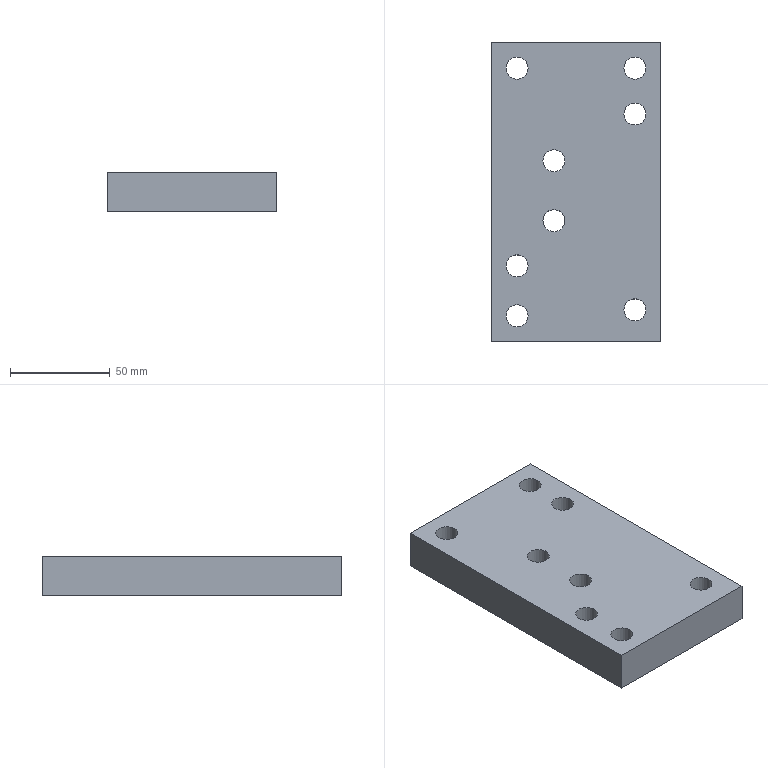Part | STEP file | 106_id3178_x_t | 1 solid | 14 faces | box 85 x 150 x 20 mm | volume 239795 mm3 | cylinder 8 | plane 6 | commonest cylinder face diameters 11 x8
STEP:
#1=CARTESIAN_POINT('',(0.,0.,0.));
#2=DIRECTION('',(0.,0.,1.));
#3=DIRECTION('',(1.,0.,0.));
#4=AXIS2_PLACEMENT_3D('',#1,#2,#3);
#5=CARTESIAN_POINT('',(-565.5,-67.,105.));
#6=VERTEX_POINT('',#5);
#7=CARTESIAN_POINT('',(-571.,-67.,105.));
#8=DIRECTION('',(0.,0.,-1.));
#9=DIRECTION('',(1.,0.,0.));
#10=AXIS2_PLACEMENT_3D('',#7,#8,#9);
#11=CIRCLE('',#10,5.5);
#12=CARTESIAN_POINT('',(-571.,-67.,90.));
#13=DIRECTION('',(0.,0.,1.));
#14=DIRECTION('',(-1.,0.,0.));
#15=AXIS2_PLACEMENT_3D('',#12,#13,#14);
#16=CYLINDRICAL_SURFACE('',#15,5.5);
#17=CARTESIAN_POINT('',(9.425,15.));
#18=DIRECTION('',(-1.,0.));
#19=VECTOR('',#18,1.);
#20=LINE('',#17,#19);
#21=(GEOMETRIC_REPRESENTATION_CONTEXT(2)PARAMETRIC_REPRESENTATION_CONTEXT()REPRESENTATION_CONTEXT('',''));
#22=DEFINITIONAL_REPRESENTATION('',(#20),#21);
#23=PCURVE('',#16,#22);
#24=CARTESIAN_POINT('',(-532.5,-4.,105.));
#25=DIRECTION('',(0.,0.,1.));
#26=DIRECTION('',(0.,-1.,0.));
#27=AXIS2_PLACEMENT_3D('',#24,#25,#26);
#28=PLANE('',#27);
#29=CARTESIAN_POINT('',(63.,-33.));
#30=CARTESIAN_POINT('',(72.526,-33.));
#31=CARTESIAN_POINT('',(67.763,-41.25));
#32=CARTESIAN_POINT('',(63.,-49.5));
#33=CARTESIAN_POINT('',(58.237,-41.25));
#34=CARTESIAN_POINT('',(53.474,-33.));
#35=CARTESIAN_POINT('',(63.,-33.));
#36=(BOUNDED_CURVE()B_SPLINE_CURVE(2,(#29,#30,#31,#32,#33,#34,#35),.UNSPECIFIED.,.T.,.F.)B_SPLINE_CURVE_WITH_KNOTS((1,2,2,2,2,1),(-2.094,0.,2.094,4.189,6.283,8.378),.UNSPECIFIED.)CURVE()GEOMETRIC_REPRESENTATION_ITEM()RATIONAL_B_SPLINE_CURVE((1.,0.5,1.,0.5,1.,0.5,1.))REPRESENTATION_ITEM(''));
#37=(GEOMETRIC_REPRESENTATION_CONTEXT(2)PARAMETRIC_REPRESENTATION_CONTEXT()REPRESENTATION_CONTEXT('',''));
#38=DEFINITIONAL_REPRESENTATION('',(#36),#37);
#39=PCURVE('',#28,#38);
#40=SURFACE_CURVE('',#11,(#23,#39),.PCURVE_S1.);
#41=EDGE_CURVE('',#6,#6,#40,.T.);
#42=ORIENTED_EDGE('',*,*,#41,.T.);
#43=CARTESIAN_POINT('',(-565.5,-67.,85.));
#44=VERTEX_POINT('',#43);
#45=CARTESIAN_POINT('',(-565.5,-67.,85.));
#46=CARTESIAN_POINT('',(-565.5,-67.,105.));
#47=B_SPLINE_CURVE_WITH_KNOTS('',1,(#45,#46),.UNSPECIFIED.,.F.,.F.,(2,2),(-5.,15.),.PIECEWISE_BEZIER_KNOTS.);
#48=CARTESIAN_POINT('',(3.142,0.));
#49=DIRECTION('',(0.,1.));
#50=VECTOR('',#49,1.);
#51=LINE('',#48,#50);
#52=(GEOMETRIC_REPRESENTATION_CONTEXT(2)PARAMETRIC_REPRESENTATION_CONTEXT()REPRESENTATION_CONTEXT('',''));
#53=DEFINITIONAL_REPRESENTATION('',(#51),#52);
#54=PCURVE('',#16,#53);
#55=CARTESIAN_POINT('',(9.425,0.));
#56=DIRECTION('',(0.,1.));
#57=VECTOR('',#56,1.);
#58=LINE('',#55,#57);
#59=(GEOMETRIC_REPRESENTATION_CONTEXT(2)PARAMETRIC_REPRESENTATION_CONTEXT()REPRESENTATION_CONTEXT('',''));
#60=DEFINITIONAL_REPRESENTATION('',(#58),#59);
#61=PCURVE('',#16,#60);
#62=SEAM_CURVE('',#47,(#54,#61),.PCURVE_S1.);
#63=EDGE_CURVE('',#44,#6,#62,.T.);
#64=ORIENTED_EDGE('',*,*,#63,.F.);
#65=CARTESIAN_POINT('',(-571.,-67.,85.));
#66=DIRECTION('',(0.,0.,1.));
#67=DIRECTION('',(-1.,0.,0.));
#68=AXIS2_PLACEMENT_3D('',#65,#66,#67);
#69=CIRCLE('',#68,5.5);
#70=CARTESIAN_POINT('',(0.,-5.));
#71=DIRECTION('',(1.,0.));
#72=VECTOR('',#71,1.);
#73=LINE('',#70,#72);
#74=(GEOMETRIC_REPRESENTATION_CONTEXT(2)PARAMETRIC_REPRESENTATION_CONTEXT()REPRESENTATION_CONTEXT('',''));
#75=DEFINITIONAL_REPRESENTATION('',(#73),#74);
#76=PCURVE('',#16,#75);
#77=CARTESIAN_POINT('',(-532.5,-4.,85.));
#78=DIRECTION('',(0.,0.,-1.));
#79=DIRECTION('',(0.,1.,0.));
#80=AXIS2_PLACEMENT_3D('',#77,#78,#79);
#81=PLANE('',#80);
#82=CARTESIAN_POINT('',(-63.,-44.));
#83=CARTESIAN_POINT('',(-72.526,-44.));
#84=CARTESIAN_POINT('',(-67.763,-35.75));
#85=CARTESIAN_POINT('',(-63.,-27.5));
#86=CARTESIAN_POINT('',(-58.237,-35.75));
#87=CARTESIAN_POINT('',(-53.474,-44.));
#88=CARTESIAN_POINT('',(-63.,-44.));
#89=(BOUNDED_CURVE()B_SPLINE_CURVE(2,(#82,#83,#84,#85,#86,#87,#88),.UNSPECIFIED.,.T.,.F.)B_SPLINE_CURVE_WITH_KNOTS((1,2,2,2,2,1),(-2.094,0.,2.094,4.189,6.283,8.378),.UNSPECIFIED.)CURVE()GEOMETRIC_REPRESENTATION_ITEM()RATIONAL_B_SPLINE_CURVE((1.,0.5,1.,0.5,1.,0.5,1.))REPRESENTATION_ITEM(''));
#90=(GEOMETRIC_REPRESENTATION_CONTEXT(2)PARAMETRIC_REPRESENTATION_CONTEXT()REPRESENTATION_CONTEXT('',''));
#91=DEFINITIONAL_REPRESENTATION('',(#89),#90);
#92=PCURVE('',#81,#91);
#93=SURFACE_CURVE('',#69,(#76,#92),.PCURVE_S1.);
#94=EDGE_CURVE('',#44,#44,#93,.T.);
#95=ORIENTED_EDGE('',*,*,#94,.T.);
#96=ORIENTED_EDGE('',*,*,#63,.T.);
#97=EDGE_LOOP('',(#42,#64,#95,#96));
#98=FACE_BOUND('',#97,.F.);
#99=ADVANCED_FACE('',(#98),#16,.F.);
#100=CARTESIAN_POINT('',(-506.5,57.,105.));
#101=VERTEX_POINT('',#100);
#102=CARTESIAN_POINT('',(-512.,57.,105.));
#103=DIRECTION('',(0.,0.,-1.));
#104=DIRECTION('',(1.,0.,0.));
#105=AXIS2_PLACEMENT_3D('',#102,#103,#104);
#106=CIRCLE('',#105,5.5);
#107=CARTESIAN_POINT('',(-512.,57.,90.));
#108=DIRECTION('',(0.,0.,1.));
#109=DIRECTION('',(-1.,0.,0.));
#110=AXIS2_PLACEMENT_3D('',#107,#108,#109);
#111=CYLINDRICAL_SURFACE('',#110,5.5);
#112=CARTESIAN_POINT('',(9.425,15.));
#113=DIRECTION('',(-1.,0.));
#114=VECTOR('',#113,1.);
#115=LINE('',#112,#114);
#116=(GEOMETRIC_REPRESENTATION_CONTEXT(2)PARAMETRIC_REPRESENTATION_CONTEXT()REPRESENTATION_CONTEXT('',''));
#117=DEFINITIONAL_REPRESENTATION('',(#115),#116);
#118=PCURVE('',#111,#117);
#119=CARTESIAN_POINT('',(-61.,26.));
#120=CARTESIAN_POINT('',(-51.474,26.));
#121=CARTESIAN_POINT('',(-56.237,17.75));
#122=CARTESIAN_POINT('',(-61.,9.5));
#123=CARTESIAN_POINT('',(-65.763,17.75));
#124=CARTESIAN_POINT('',(-70.526,26.));
#125=CARTESIAN_POINT('',(-61.,26.));
#126=(BOUNDED_CURVE()B_SPLINE_CURVE(2,(#119,#120,#121,#122,#123,#124,#125),.UNSPECIFIED.,.T.,.F.)B_SPLINE_CURVE_WITH_KNOTS((1,2,2,2,2,1),(-2.094,0.,2.094,4.189,6.283,8.378),.UNSPECIFIED.)CURVE()GEOMETRIC_REPRESENTATION_ITEM()RATIONAL_B_SPLINE_CURVE((1.,0.5,1.,0.5,1.,0.5,1.))REPRESENTATION_ITEM(''));
#127=(GEOMETRIC_REPRESENTATION_CONTEXT(2)PARAMETRIC_REPRESENTATION_CONTEXT()REPRESENTATION_CONTEXT('',''));
#128=DEFINITIONAL_REPRESENTATION('',(#126),#127);
#129=PCURVE('',#28,#128);
#130=SURFACE_CURVE('',#106,(#118,#129),.PCURVE_S1.);
#131=EDGE_CURVE('',#101,#101,#130,.T.);
#132=ORIENTED_EDGE('',*,*,#131,.T.);
#133=CARTESIAN_POINT('',(-506.5,57.,85.));
#134=VERTEX_POINT('',#133);
#135=CARTESIAN_POINT('',(-506.5,57.,85.));
#136=CARTESIAN_POINT('',(-506.5,57.,105.));
#137=B_SPLINE_CURVE_WITH_KNOTS('',1,(#135,#136),.UNSPECIFIED.,.F.,.F.,(2,2),(-5.,15.),.PIECEWISE_BEZIER_KNOTS.);
#138=CARTESIAN_POINT('',(3.142,0.));
#139=DIRECTION('',(0.,1.));
#140=VECTOR('',#139,1.);
#141=LINE('',#138,#140);
#142=(GEOMETRIC_REPRESENTATION_CONTEXT(2)PARAMETRIC_REPRESENTATION_CONTEXT()REPRESENTATION_CONTEXT('',''));
#143=DEFINITIONAL_REPRESENTATION('',(#141),#142);
#144=PCURVE('',#111,#143);
#145=CARTESIAN_POINT('',(9.425,0.));
#146=DIRECTION('',(0.,1.));
#147=VECTOR('',#146,1.);
#148=LINE('',#145,#147);
#149=(GEOMETRIC_REPRESENTATION_CONTEXT(2)PARAMETRIC_REPRESENTATION_CONTEXT()REPRESENTATION_CONTEXT('',''));
#150=DEFINITIONAL_REPRESENTATION('',(#148),#149);
#151=PCURVE('',#111,#150);
#152=SEAM_CURVE('',#137,(#144,#151),.PCURVE_S1.);
#153=EDGE_CURVE('',#134,#101,#152,.T.);
#154=ORIENTED_EDGE('',*,*,#153,.F.);
#155=CARTESIAN_POINT('',(-512.,57.,85.));
#156=DIRECTION('',(0.,0.,1.));
#157=DIRECTION('',(-1.,0.,0.));
#158=AXIS2_PLACEMENT_3D('',#155,#156,#157);
#159=CIRCLE('',#158,5.5);
#160=CARTESIAN_POINT('',(0.,-5.));
#161=DIRECTION('',(1.,0.));
#162=VECTOR('',#161,1.);
#163=LINE('',#160,#162);
#164=(GEOMETRIC_REPRESENTATION_CONTEXT(2)PARAMETRIC_REPRESENTATION_CONTEXT()REPRESENTATION_CONTEXT('',''));
#165=DEFINITIONAL_REPRESENTATION('',(#163),#164);
#166=PCURVE('',#111,#165);
#167=CARTESIAN_POINT('',(61.,15.));
#168=CARTESIAN_POINT('',(51.474,15.));
#169=CARTESIAN_POINT('',(56.237,23.25));
#170=CARTESIAN_POINT('',(61.,31.5));
#171=CARTESIAN_POINT('',(65.763,23.25));
#172=CARTESIAN_POINT('',(70.526,15.));
#173=CARTESIAN_POINT('',(61.,15.));
#174=(BOUNDED_CURVE()B_SPLINE_CURVE(2,(#167,#168,#169,#170,#171,#172,#173),.UNSPECIFIED.,.T.,.F.)B_SPLINE_CURVE_WITH_KNOTS((1,2,2,2,2,1),(-2.094,0.,2.094,4.189,6.283,8.378),.UNSPECIFIED.)CURVE()GEOMETRIC_REPRESENTATION_ITEM()RATIONAL_B_SPLINE_CURVE((1.,0.5,1.,0.5,1.,0.5,1.))REPRESENTATION_ITEM(''));
#175=(GEOMETRIC_REPRESENTATION_CONTEXT(2)PARAMETRIC_REPRESENTATION_CONTEXT()REPRESENTATION_CONTEXT('',''));
#176=DEFINITIONAL_REPRESENTATION('',(#174),#175);
#177=PCURVE('',#81,#176);
#178=SURFACE_CURVE('',#159,(#166,#177),.PCURVE_S1.);
#179=EDGE_CURVE('',#134,#134,#178,.T.);
#180=ORIENTED_EDGE('',*,*,#179,.T.);
#181=ORIENTED_EDGE('',*,*,#153,.T.);
#182=EDGE_LOOP('',(#132,#154,#180,#181));
#183=FACE_BOUND('',#182,.F.);
#184=ADVANCED_FACE('',(#183),#111,.F.);
#185=CARTESIAN_POINT('',(-584.,-80.,85.));
#186=VERTEX_POINT('',#185);
#187=CARTESIAN_POINT('',(-584.,-80.,105.));
#188=VERTEX_POINT('',#187);
#189=CARTESIAN_POINT('',(-584.,-80.,90.));
#190=DIRECTION('',(0.,0.,1.));
#191=VECTOR('',#190,1.);
#192=LINE('',#189,#191);
#193=CARTESIAN_POINT('',(-584.,-4.,90.));
#194=DIRECTION('',(-1.,0.,0.));
#195=DIRECTION('',(0.,0.,-1.));
#196=AXIS2_PLACEMENT_3D('',#193,#194,#195);
#197=PLANE('',#196);
#198=CARTESIAN_POINT('',(0.,76.));
#199=DIRECTION('',(-1.,0.));
#200=VECTOR('',#199,1.);
#201=LINE('',#198,#200);
#202=(GEOMETRIC_REPRESENTATION_CONTEXT(2)PARAMETRIC_REPRESENTATION_CONTEXT()REPRESENTATION_CONTEXT('',''));
#203=DEFINITIONAL_REPRESENTATION('',(#201),#202);
#204=PCURVE('',#197,#203);
#205=CARTESIAN_POINT('',(-532.5,-80.,90.));
#206=DIRECTION('',(0.,-1.,0.));
#207=DIRECTION('',(0.,0.,-1.));
#208=AXIS2_PLACEMENT_3D('',#205,#206,#207);
#209=PLANE('',#208);
#210=CARTESIAN_POINT('',(0.,-51.5));
#211=DIRECTION('',(-1.,0.));
#212=VECTOR('',#211,1.);
#213=LINE('',#210,#212);
#214=(GEOMETRIC_REPRESENTATION_CONTEXT(2)PARAMETRIC_REPRESENTATION_CONTEXT()REPRESENTATION_CONTEXT('',''));
#215=DEFINITIONAL_REPRESENTATION('',(#213),#214);
#216=PCURVE('',#209,#215);
#217=SURFACE_CURVE('',#192,(#204,#216),.PCURVE_S1.);
#218=EDGE_CURVE('',#186,#188,#217,.T.);
#219=ORIENTED_EDGE('',*,*,#218,.T.);
#220=CARTESIAN_POINT('',(-584.,70.,105.));
#221=VERTEX_POINT('',#220);
#222=CARTESIAN_POINT('',(-584.,-4.,105.));
#223=DIRECTION('',(0.,1.,0.));
#224=VECTOR('',#223,1.);
#225=LINE('',#222,#224);
#226=CARTESIAN_POINT('',(-15.,0.));
#227=DIRECTION('',(0.,-1.));
#228=VECTOR('',#227,1.);
#229=LINE('',#226,#228);
#230=(GEOMETRIC_REPRESENTATION_CONTEXT(2)PARAMETRIC_REPRESENTATION_CONTEXT()REPRESENTATION_CONTEXT('',''));
#231=DEFINITIONAL_REPRESENTATION('',(#229),#230);
#232=PCURVE('',#197,#231);
#233=CARTESIAN_POINT('',(0.,-51.5));
#234=DIRECTION('',(-1.,0.));
#235=VECTOR('',#234,1.);
#236=LINE('',#233,#235);
#237=(GEOMETRIC_REPRESENTATION_CONTEXT(2)PARAMETRIC_REPRESENTATION_CONTEXT()REPRESENTATION_CONTEXT('',''));
#238=DEFINITIONAL_REPRESENTATION('',(#236),#237);
#239=PCURVE('',#28,#238);
#240=SURFACE_CURVE('',#225,(#232,#239),.PCURVE_S1.);
#241=EDGE_CURVE('',#188,#221,#240,.T.);
#242=ORIENTED_EDGE('',*,*,#241,.T.);
#243=CARTESIAN_POINT('',(-584.,70.,85.));
#244=VERTEX_POINT('',#243);
#245=CARTESIAN_POINT('',(-584.,70.,90.));
#246=DIRECTION('',(0.,0.,1.));
#247=VECTOR('',#246,1.);
#248=LINE('',#245,#247);
#249=CARTESIAN_POINT('',(0.,-74.));
#250=DIRECTION('',(-1.,0.));
#251=VECTOR('',#250,1.);
#252=LINE('',#249,#251);
#253=(GEOMETRIC_REPRESENTATION_CONTEXT(2)PARAMETRIC_REPRESENTATION_CONTEXT()REPRESENTATION_CONTEXT('',''));
#254=DEFINITIONAL_REPRESENTATION('',(#252),#253);
#255=PCURVE('',#197,#254);
#256=CARTESIAN_POINT('',(-532.5,70.,90.));
#257=DIRECTION('',(0.,1.,0.));
#258=DIRECTION('',(0.,0.,1.));
#259=AXIS2_PLACEMENT_3D('',#256,#257,#258);
#260=PLANE('',#259);
#261=CARTESIAN_POINT('',(0.,-51.5));
#262=DIRECTION('',(1.,0.));
#263=VECTOR('',#262,1.);
#264=LINE('',#261,#263);
#265=(GEOMETRIC_REPRESENTATION_CONTEXT(2)PARAMETRIC_REPRESENTATION_CONTEXT()REPRESENTATION_CONTEXT('',''));
#266=DEFINITIONAL_REPRESENTATION('',(#264),#265);
#267=PCURVE('',#260,#266);
#268=SURFACE_CURVE('',#248,(#255,#267),.PCURVE_S1.);
#269=EDGE_CURVE('',#244,#221,#268,.T.);
#270=ORIENTED_EDGE('',*,*,#269,.F.);
#271=CARTESIAN_POINT('',(-584.,-4.,85.));
#272=DIRECTION('',(0.,-1.,0.));
#273=VECTOR('',#272,1.);
#274=LINE('',#271,#273);
#275=CARTESIAN_POINT('',(5.,0.));
#276=DIRECTION('',(0.,1.));
#277=VECTOR('',#276,1.);
#278=LINE('',#275,#277);
#279=(GEOMETRIC_REPRESENTATION_CONTEXT(2)PARAMETRIC_REPRESENTATION_CONTEXT()REPRESENTATION_CONTEXT('',''));
#280=DEFINITIONAL_REPRESENTATION('',(#278),#279);
#281=PCURVE('',#197,#280);
#282=CARTESIAN_POINT('',(0.,-51.5));
#283=DIRECTION('',(-1.,0.));
#284=VECTOR('',#283,1.);
#285=LINE('',#282,#284);
#286=(GEOMETRIC_REPRESENTATION_CONTEXT(2)PARAMETRIC_REPRESENTATION_CONTEXT()REPRESENTATION_CONTEXT('',''));
#287=DEFINITIONAL_REPRESENTATION('',(#285),#286);
#288=PCURVE('',#81,#287);
#289=SURFACE_CURVE('',#274,(#281,#288),.PCURVE_S1.);
#290=EDGE_CURVE('',#244,#186,#289,.T.);
#291=ORIENTED_EDGE('',*,*,#290,.T.);
#292=EDGE_LOOP('',(#219,#242,#270,#291));
#293=FACE_BOUND('',#292,.T.);
#294=ADVANCED_FACE('',(#293),#197,.T.);
#295=CARTESIAN_POINT('',(-499.,-80.,85.));
#296=VERTEX_POINT('',#295);
#297=CARTESIAN_POINT('',(-499.,-80.,105.));
#298=VERTEX_POINT('',#297);
#299=CARTESIAN_POINT('',(-499.,-80.,90.));
#300=DIRECTION('',(0.,0.,1.));
#301=VECTOR('',#300,1.);
#302=LINE('',#299,#301);
#303=CARTESIAN_POINT('',(0.,33.5));
#304=DIRECTION('',(-1.,0.));
#305=VECTOR('',#304,1.);
#306=LINE('',#303,#305);
#307=(GEOMETRIC_REPRESENTATION_CONTEXT(2)PARAMETRIC_REPRESENTATION_CONTEXT()REPRESENTATION_CONTEXT('',''));
#308=DEFINITIONAL_REPRESENTATION('',(#306),#307);
#309=PCURVE('',#209,#308);
#310=CARTESIAN_POINT('',(-499.,-4.,90.));
#311=DIRECTION('',(1.,0.,0.));
#312=DIRECTION('',(0.,0.,1.));
#313=AXIS2_PLACEMENT_3D('',#310,#311,#312);
#314=PLANE('',#313);
#315=CARTESIAN_POINT('',(0.,76.));
#316=DIRECTION('',(1.,0.));
#317=VECTOR('',#316,1.);
#318=LINE('',#315,#317);
#319=(GEOMETRIC_REPRESENTATION_CONTEXT(2)PARAMETRIC_REPRESENTATION_CONTEXT()REPRESENTATION_CONTEXT('',''));
#320=DEFINITIONAL_REPRESENTATION('',(#318),#319);
#321=PCURVE('',#314,#320);
#322=SURFACE_CURVE('',#302,(#309,#321),.PCURVE_S1.);
#323=EDGE_CURVE('',#296,#298,#322,.T.);
#324=ORIENTED_EDGE('',*,*,#323,.T.);
#325=CARTESIAN_POINT('',(-532.5,-80.,105.));
#326=DIRECTION('',(-1.,0.,0.));
#327=VECTOR('',#326,1.);
#328=LINE('',#325,#327);
#329=CARTESIAN_POINT('',(-15.,0.));
#330=DIRECTION('',(0.,-1.));
#331=VECTOR('',#330,1.);
#332=LINE('',#329,#331);
#333=(GEOMETRIC_REPRESENTATION_CONTEXT(2)PARAMETRIC_REPRESENTATION_CONTEXT()REPRESENTATION_CONTEXT('',''));
#334=DEFINITIONAL_REPRESENTATION('',(#332),#333);
#335=PCURVE('',#209,#334);
#336=CARTESIAN_POINT('',(76.,0.));
#337=DIRECTION('',(0.,-1.));
#338=VECTOR('',#337,1.);
#339=LINE('',#336,#338);
#340=(GEOMETRIC_REPRESENTATION_CONTEXT(2)PARAMETRIC_REPRESENTATION_CONTEXT()REPRESENTATION_CONTEXT('',''));
#341=DEFINITIONAL_REPRESENTATION('',(#339),#340);
#342=PCURVE('',#28,#341);
#343=SURFACE_CURVE('',#328,(#335,#342),.PCURVE_S1.);
#344=EDGE_CURVE('',#298,#188,#343,.T.);
#345=ORIENTED_EDGE('',*,*,#344,.T.);
#346=ORIENTED_EDGE('',*,*,#218,.F.);
#347=CARTESIAN_POINT('',(-532.5,-80.,85.));
#348=DIRECTION('',(1.,0.,0.));
#349=VECTOR('',#348,1.);
#350=LINE('',#347,#349);
#351=CARTESIAN_POINT('',(5.,0.));
#352=DIRECTION('',(0.,1.));
#353=VECTOR('',#352,1.);
#354=LINE('',#351,#353);
#355=(GEOMETRIC_REPRESENTATION_CONTEXT(2)PARAMETRIC_REPRESENTATION_CONTEXT()REPRESENTATION_CONTEXT('',''));
#356=DEFINITIONAL_REPRESENTATION('',(#354),#355);
#357=PCURVE('',#209,#356);
#358=CARTESIAN_POINT('',(-76.,0.));
#359=DIRECTION('',(0.,1.));
#360=VECTOR('',#359,1.);
#361=LINE('',#358,#360);
#362=(GEOMETRIC_REPRESENTATION_CONTEXT(2)PARAMETRIC_REPRESENTATION_CONTEXT()REPRESENTATION_CONTEXT('',''));
#363=DEFINITIONAL_REPRESENTATION('',(#361),#362);
#364=PCURVE('',#81,#363);
#365=SURFACE_CURVE('',#350,(#357,#364),.PCURVE_S1.);
#366=EDGE_CURVE('',#186,#296,#365,.T.);
#367=ORIENTED_EDGE('',*,*,#366,.T.);
#368=EDGE_LOOP('',(#324,#345,#346,#367));
#369=FACE_BOUND('',#368,.T.);
#370=ADVANCED_FACE('',(#369),#209,.T.);
#371=CARTESIAN_POINT('',(-499.,70.,85.));
#372=VERTEX_POINT('',#371);
#373=CARTESIAN_POINT('',(-499.,70.,105.));
#374=VERTEX_POINT('',#373);
#375=CARTESIAN_POINT('',(-499.,70.,90.));
#376=DIRECTION('',(0.,0.,1.));
#377=VECTOR('',#376,1.);
#378=LINE('',#375,#377);
#379=CARTESIAN_POINT('',(0.,-74.));
#380=DIRECTION('',(1.,0.));
#381=VECTOR('',#380,1.);
#382=LINE('',#379,#381);
#383=(GEOMETRIC_REPRESENTATION_CONTEXT(2)PARAMETRIC_REPRESENTATION_CONTEXT()REPRESENTATION_CONTEXT('',''));
#384=DEFINITIONAL_REPRESENTATION('',(#382),#383);
#385=PCURVE('',#314,#384);
#386=CARTESIAN_POINT('',(0.,33.5));
#387=DIRECTION('',(1.,0.));
#388=VECTOR('',#387,1.);
#389=LINE('',#386,#388);
#390=(GEOMETRIC_REPRESENTATION_CONTEXT(2)PARAMETRIC_REPRESENTATION_CONTEXT()REPRESENTATION_CONTEXT('',''));
#391=DEFINITIONAL_REPRESENTATION('',(#389),#390);
#392=PCURVE('',#260,#391);
#393=SURFACE_CURVE('',#378,(#385,#392),.PCURVE_S1.);
#394=EDGE_CURVE('',#372,#374,#393,.T.);
#395=ORIENTED_EDGE('',*,*,#394,.T.);
#396=CARTESIAN_POINT('',(-499.,-4.,105.));
#397=DIRECTION('',(0.,-1.,0.));
#398=VECTOR('',#397,1.);
#399=LINE('',#396,#398);
#400=CARTESIAN_POINT('',(15.,0.));
#401=DIRECTION('',(0.,1.));
#402=VECTOR('',#401,1.);
#403=LINE('',#400,#402);
#404=(GEOMETRIC_REPRESENTATION_CONTEXT(2)PARAMETRIC_REPRESENTATION_CONTEXT()REPRESENTATION_CONTEXT('',''));
#405=DEFINITIONAL_REPRESENTATION('',(#403),#404);
#406=PCURVE('',#314,#405);
#407=CARTESIAN_POINT('',(0.,33.5));
#408=DIRECTION('',(1.,0.));
#409=VECTOR('',#408,1.);
#410=LINE('',#407,#409);
#411=(GEOMETRIC_REPRESENTATION_CONTEXT(2)PARAMETRIC_REPRESENTATION_CONTEXT()REPRESENTATION_CONTEXT('',''));
#412=DEFINITIONAL_REPRESENTATION('',(#410),#411);
#413=PCURVE('',#28,#412);
#414=SURFACE_CURVE('',#399,(#406,#413),.PCURVE_S1.);
#415=EDGE_CURVE('',#374,#298,#414,.T.);
#416=ORIENTED_EDGE('',*,*,#415,.T.);
#417=ORIENTED_EDGE('',*,*,#323,.F.);
#418=CARTESIAN_POINT('',(-499.,-4.,85.));
#419=DIRECTION('',(0.,1.,0.));
#420=VECTOR('',#419,1.);
#421=LINE('',#418,#420);
#422=CARTESIAN_POINT('',(-5.,0.));
#423=DIRECTION('',(0.,-1.));
#424=VECTOR('',#423,1.);
#425=LINE('',#422,#424);
#426=(GEOMETRIC_REPRESENTATION_CONTEXT(2)PARAMETRIC_REPRESENTATION_CONTEXT()REPRESENTATION_CONTEXT('',''));
#427=DEFINITIONAL_REPRESENTATION('',(#425),#426);
#428=PCURVE('',#314,#427);
#429=CARTESIAN_POINT('',(0.,33.5));
#430=DIRECTION('',(1.,0.));
#431=VECTOR('',#430,1.);
#432=LINE('',#429,#431);
#433=(GEOMETRIC_REPRESENTATION_CONTEXT(2)PARAMETRIC_REPRESENTATION_CONTEXT()REPRESENTATION_CONTEXT('',''));
#434=DEFINITIONAL_REPRESENTATION('',(#432),#433);
#435=PCURVE('',#81,#434);
#436=SURFACE_CURVE('',#421,(#428,#435),.PCURVE_S1.);
#437=EDGE_CURVE('',#296,#372,#436,.T.);
#438=ORIENTED_EDGE('',*,*,#437,.T.);
#439=EDGE_LOOP('',(#395,#416,#417,#438));
#440=FACE_BOUND('',#439,.T.);
#441=ADVANCED_FACE('',(#440),#314,.T.);
#442=CARTESIAN_POINT('',(-532.5,70.,85.));
#443=DIRECTION('',(-1.,0.,0.));
#444=VECTOR('',#443,1.);
#445=LINE('',#442,#444);
#446=CARTESIAN_POINT('',(-5.,0.));
#447=DIRECTION('',(0.,-1.));
#448=VECTOR('',#447,1.);
#449=LINE('',#446,#448);
#450=(GEOMETRIC_REPRESENTATION_CONTEXT(2)PARAMETRIC_REPRESENTATION_CONTEXT()REPRESENTATION_CONTEXT('',''));
#451=DEFINITIONAL_REPRESENTATION('',(#449),#450);
#452=PCURVE('',#260,#451);
#453=CARTESIAN_POINT('',(74.,0.));
#454=DIRECTION('',(0.,-1.));
#455=VECTOR('',#454,1.);
#456=LINE('',#453,#455);
#457=(GEOMETRIC_REPRESENTATION_CONTEXT(2)PARAMETRIC_REPRESENTATION_CONTEXT()REPRESENTATION_CONTEXT('',''));
#458=DEFINITIONAL_REPRESENTATION('',(#456),#457);
#459=PCURVE('',#81,#458);
#460=SURFACE_CURVE('',#445,(#452,#459),.PCURVE_S1.);
#461=EDGE_CURVE('',#372,#244,#460,.T.);
#462=ORIENTED_EDGE('',*,*,#461,.T.);
#463=ORIENTED_EDGE('',*,*,#269,.T.);
#464=CARTESIAN_POINT('',(-532.5,70.,105.));
#465=DIRECTION('',(1.,0.,0.));
#466=VECTOR('',#465,1.);
#467=LINE('',#464,#466);
#468=CARTESIAN_POINT('',(15.,0.));
#469=DIRECTION('',(0.,1.));
#470=VECTOR('',#469,1.);
#471=LINE('',#468,#470);
#472=(GEOMETRIC_REPRESENTATION_CONTEXT(2)PARAMETRIC_REPRESENTATION_CONTEXT()REPRESENTATION_CONTEXT('',''));
#473=DEFINITIONAL_REPRESENTATION('',(#471),#472);
#474=PCURVE('',#260,#473);
#475=CARTESIAN_POINT('',(-74.,0.));
#476=DIRECTION('',(0.,1.));
#477=VECTOR('',#476,1.);
#478=LINE('',#475,#477);
#479=(GEOMETRIC_REPRESENTATION_CONTEXT(2)PARAMETRIC_REPRESENTATION_CONTEXT()REPRESENTATION_CONTEXT('',''));
#480=DEFINITIONAL_REPRESENTATION('',(#478),#479);
#481=PCURVE('',#28,#480);
#482=SURFACE_CURVE('',#467,(#474,#481),.PCURVE_S1.);
#483=EDGE_CURVE('',#221,#374,#482,.T.);
#484=ORIENTED_EDGE('',*,*,#483,.T.);
#485=ORIENTED_EDGE('',*,*,#394,.F.);
#486=EDGE_LOOP('',(#462,#463,#484,#485));
#487=FACE_BOUND('',#486,.T.);
#488=ADVANCED_FACE('',(#487),#260,.T.);
#489=CARTESIAN_POINT('',(-506.5,-64.,105.));
#490=VERTEX_POINT('',#489);
#491=CARTESIAN_POINT('',(-512.,-64.,105.));
#492=DIRECTION('',(0.,0.,-1.));
#493=DIRECTION('',(1.,0.,0.));
#494=AXIS2_PLACEMENT_3D('',#491,#492,#493);
#495=CIRCLE('',#494,5.5);
#496=CARTESIAN_POINT('',(-512.,-64.,90.));
#497=DIRECTION('',(0.,0.,1.));
#498=DIRECTION('',(-1.,0.,0.));
#499=AXIS2_PLACEMENT_3D('',#496,#497,#498);
#500=CYLINDRICAL_SURFACE('',#499,5.5);
#501=CARTESIAN_POINT('',(9.425,15.));
#502=DIRECTION('',(-1.,0.));
#503=VECTOR('',#502,1.);
#504=LINE('',#501,#503);
#505=(GEOMETRIC_REPRESENTATION_CONTEXT(2)PARAMETRIC_REPRESENTATION_CONTEXT()REPRESENTATION_CONTEXT('',''));
#506=DEFINITIONAL_REPRESENTATION('',(#504),#505);
#507=PCURVE('',#500,#506);
#508=CARTESIAN_POINT('',(60.,26.));
#509=CARTESIAN_POINT('',(69.526,26.));
#510=CARTESIAN_POINT('',(64.763,17.75));
#511=CARTESIAN_POINT('',(60.,9.5));
#512=CARTESIAN_POINT('',(55.237,17.75));
#513=CARTESIAN_POINT('',(50.474,26.));
#514=CARTESIAN_POINT('',(60.,26.));
#515=(BOUNDED_CURVE()B_SPLINE_CURVE(2,(#508,#509,#510,#511,#512,#513,#514),.UNSPECIFIED.,.T.,.F.)B_SPLINE_CURVE_WITH_KNOTS((1,2,2,2,2,1),(-2.094,0.,2.094,4.189,6.283,8.378),.UNSPECIFIED.)CURVE()GEOMETRIC_REPRESENTATION_ITEM()RATIONAL_B_SPLINE_CURVE((1.,0.5,1.,0.5,1.,0.5,1.))REPRESENTATION_ITEM(''));
#516=(GEOMETRIC_REPRESENTATION_CONTEXT(2)PARAMETRIC_REPRESENTATION_CONTEXT()REPRESENTATION_CONTEXT('',''));
#517=DEFINITIONAL_REPRESENTATION('',(#515),#516);
#518=PCURVE('',#28,#517);
#519=SURFACE_CURVE('',#495,(#507,#518),.PCURVE_S1.);
#520=EDGE_CURVE('',#490,#490,#519,.T.);
#521=ORIENTED_EDGE('',*,*,#520,.T.);
#522=CARTESIAN_POINT('',(-506.5,-64.,85.));
#523=VERTEX_POINT('',#522);
#524=CARTESIAN_POINT('',(-506.5,-64.,85.));
#525=CARTESIAN_POINT('',(-506.5,-64.,105.));
#526=B_SPLINE_CURVE_WITH_KNOTS('',1,(#524,#525),.UNSPECIFIED.,.F.,.F.,(2,2),(-5.,15.),.PIECEWISE_BEZIER_KNOTS.);
#527=CARTESIAN_POINT('',(3.142,0.));
#528=DIRECTION('',(0.,1.));
#529=VECTOR('',#528,1.);
#530=LINE('',#527,#529);
#531=(GEOMETRIC_REPRESENTATION_CONTEXT(2)PARAMETRIC_REPRESENTATION_CONTEXT()REPRESENTATION_CONTEXT('',''));
#532=DEFINITIONAL_REPRESENTATION('',(#530),#531);
#533=PCURVE('',#500,#532);
#534=CARTESIAN_POINT('',(9.425,0.));
#535=DIRECTION('',(0.,1.));
#536=VECTOR('',#535,1.);
#537=LINE('',#534,#536);
#538=(GEOMETRIC_REPRESENTATION_CONTEXT(2)PARAMETRIC_REPRESENTATION_CONTEXT()REPRESENTATION_CONTEXT('',''));
#539=DEFINITIONAL_REPRESENTATION('',(#537),#538);
#540=PCURVE('',#500,#539);
#541=SEAM_CURVE('',#526,(#533,#540),.PCURVE_S1.);
#542=EDGE_CURVE('',#523,#490,#541,.T.);
#543=ORIENTED_EDGE('',*,*,#542,.F.);
#544=CARTESIAN_POINT('',(-512.,-64.,85.));
#545=DIRECTION('',(0.,0.,1.));
#546=DIRECTION('',(-1.,0.,0.));
#547=AXIS2_PLACEMENT_3D('',#544,#545,#546);
#548=CIRCLE('',#547,5.5);
#549=CARTESIAN_POINT('',(0.,-5.));
#550=DIRECTION('',(1.,0.));
#551=VECTOR('',#550,1.);
#552=LINE('',#549,#551);
#553=(GEOMETRIC_REPRESENTATION_CONTEXT(2)PARAMETRIC_REPRESENTATION_CONTEXT()REPRESENTATION_CONTEXT('',''));
#554=DEFINITIONAL_REPRESENTATION('',(#552),#553);
#555=PCURVE('',#500,#554);
#556=CARTESIAN_POINT('',(-60.,15.));
#557=CARTESIAN_POINT('',(-69.526,15.));
#558=CARTESIAN_POINT('',(-64.763,23.25));
#559=CARTESIAN_POINT('',(-60.,31.5));
#560=CARTESIAN_POINT('',(-55.237,23.25));
#561=CARTESIAN_POINT('',(-50.474,15.));
#562=CARTESIAN_POINT('',(-60.,15.));
#563=(BOUNDED_CURVE()B_SPLINE_CURVE(2,(#556,#557,#558,#559,#560,#561,#562),.UNSPECIFIED.,.T.,.F.)B_SPLINE_CURVE_WITH_KNOTS((1,2,2,2,2,1),(-2.094,0.,2.094,4.189,6.283,8.378),.UNSPECIFIED.)CURVE()GEOMETRIC_REPRESENTATION_ITEM()RATIONAL_B_SPLINE_CURVE((1.,0.5,1.,0.5,1.,0.5,1.))REPRESENTATION_ITEM(''));
#564=(GEOMETRIC_REPRESENTATION_CONTEXT(2)PARAMETRIC_REPRESENTATION_CONTEXT()REPRESENTATION_CONTEXT('',''));
#565=DEFINITIONAL_REPRESENTATION('',(#563),#564);
#566=PCURVE('',#81,#565);
#567=SURFACE_CURVE('',#548,(#555,#566),.PCURVE_S1.);
#568=EDGE_CURVE('',#523,#523,#567,.T.);
#569=ORIENTED_EDGE('',*,*,#568,.T.);
#570=ORIENTED_EDGE('',*,*,#542,.T.);
#571=EDGE_LOOP('',(#521,#543,#569,#570));
#572=FACE_BOUND('',#571,.F.);
#573=ADVANCED_FACE('',(#572),#500,.F.);
#574=CARTESIAN_POINT('',(-565.5,57.,105.));
#575=VERTEX_POINT('',#574);
#576=CARTESIAN_POINT('',(-571.,57.,105.));
#577=DIRECTION('',(0.,0.,-1.));
#578=DIRECTION('',(1.,0.,0.));
#579=AXIS2_PLACEMENT_3D('',#576,#577,#578);
#580=CIRCLE('',#579,5.5);
#581=CARTESIAN_POINT('',(-571.,57.,90.));
#582=DIRECTION('',(0.,0.,1.));
#583=DIRECTION('',(-1.,0.,0.));
#584=AXIS2_PLACEMENT_3D('',#581,#582,#583);
#585=CYLINDRICAL_SURFACE('',#584,5.5);
#586=CARTESIAN_POINT('',(9.425,15.));
#587=DIRECTION('',(-1.,0.));
#588=VECTOR('',#587,1.);
#589=LINE('',#586,#588);
#590=(GEOMETRIC_REPRESENTATION_CONTEXT(2)PARAMETRIC_REPRESENTATION_CONTEXT()REPRESENTATION_CONTEXT('',''));
#591=DEFINITIONAL_REPRESENTATION('',(#589),#590);
#592=PCURVE('',#585,#591);
#593=CARTESIAN_POINT('',(-61.,-33.));
#594=CARTESIAN_POINT('',(-51.474,-33.));
#595=CARTESIAN_POINT('',(-56.237,-41.25));
#596=CARTESIAN_POINT('',(-61.,-49.5));
#597=CARTESIAN_POINT('',(-65.763,-41.25));
#598=CARTESIAN_POINT('',(-70.526,-33.));
#599=CARTESIAN_POINT('',(-61.,-33.));
#600=(BOUNDED_CURVE()B_SPLINE_CURVE(2,(#593,#594,#595,#596,#597,#598,#599),.UNSPECIFIED.,.T.,.F.)B_SPLINE_CURVE_WITH_KNOTS((1,2,2,2,2,1),(-2.094,0.,2.094,4.189,6.283,8.378),.UNSPECIFIED.)CURVE()GEOMETRIC_REPRESENTATION_ITEM()RATIONAL_B_SPLINE_CURVE((1.,0.5,1.,0.5,1.,0.5,1.))REPRESENTATION_ITEM(''));
#601=(GEOMETRIC_REPRESENTATION_CONTEXT(2)PARAMETRIC_REPRESENTATION_CONTEXT()REPRESENTATION_CONTEXT('',''));
#602=DEFINITIONAL_REPRESENTATION('',(#600),#601);
#603=PCURVE('',#28,#602);
#604=SURFACE_CURVE('',#580,(#592,#603),.PCURVE_S1.);
#605=EDGE_CURVE('',#575,#575,#604,.T.);
#606=ORIENTED_EDGE('',*,*,#605,.T.);
#607=CARTESIAN_POINT('',(-565.5,57.,85.));
#608=VERTEX_POINT('',#607);
#609=CARTESIAN_POINT('',(-565.5,57.,85.));
#610=CARTESIAN_POINT('',(-565.5,57.,105.));
#611=B_SPLINE_CURVE_WITH_KNOTS('',1,(#609,#610),.UNSPECIFIED.,.F.,.F.,(2,2),(-5.,15.),.PIECEWISE_BEZIER_KNOTS.);
#612=CARTESIAN_POINT('',(3.142,0.));
#613=DIRECTION('',(0.,1.));
#614=VECTOR('',#613,1.);
#615=LINE('',#612,#614);
#616=(GEOMETRIC_REPRESENTATION_CONTEXT(2)PARAMETRIC_REPRESENTATION_CONTEXT()REPRESENTATION_CONTEXT('',''));
#617=DEFINITIONAL_REPRESENTATION('',(#615),#616);
#618=PCURVE('',#585,#617);
#619=CARTESIAN_POINT('',(9.425,0.));
#620=DIRECTION('',(0.,1.));
#621=VECTOR('',#620,1.);
#622=LINE('',#619,#621);
#623=(GEOMETRIC_REPRESENTATION_CONTEXT(2)PARAMETRIC_REPRESENTATION_CONTEXT()REPRESENTATION_CONTEXT('',''));
#624=DEFINITIONAL_REPRESENTATION('',(#622),#623);
#625=PCURVE('',#585,#624);
#626=SEAM_CURVE('',#611,(#618,#625),.PCURVE_S1.);
#627=EDGE_CURVE('',#608,#575,#626,.T.);
#628=ORIENTED_EDGE('',*,*,#627,.F.);
#629=CARTESIAN_POINT('',(-571.,57.,85.));
#630=DIRECTION('',(0.,0.,1.));
#631=DIRECTION('',(-1.,0.,0.));
#632=AXIS2_PLACEMENT_3D('',#629,#630,#631);
#633=CIRCLE('',#632,5.5);
#634=CARTESIAN_POINT('',(0.,-5.));
#635=DIRECTION('',(1.,0.));
#636=VECTOR('',#635,1.);
#637=LINE('',#634,#636);
#638=(GEOMETRIC_REPRESENTATION_CONTEXT(2)PARAMETRIC_REPRESENTATION_CONTEXT()REPRESENTATION_CONTEXT('',''));
#639=DEFINITIONAL_REPRESENTATION('',(#637),#638);
#640=PCURVE('',#585,#639);
#641=CARTESIAN_POINT('',(61.,-44.));
#642=CARTESIAN_POINT('',(51.474,-44.));
#643=CARTESIAN_POINT('',(56.237,-35.75));
#644=CARTESIAN_POINT('',(61.,-27.5));
#645=CARTESIAN_POINT('',(65.763,-35.75));
#646=CARTESIAN_POINT('',(70.526,-44.));
#647=CARTESIAN_POINT('',(61.,-44.));
#648=(BOUNDED_CURVE()B_SPLINE_CURVE(2,(#641,#642,#643,#644,#645,#646,#647),.UNSPECIFIED.,.T.,.F.)B_SPLINE_CURVE_WITH_KNOTS((1,2,2,2,2,1),(-2.094,0.,2.094,4.189,6.283,8.378),.UNSPECIFIED.)CURVE()GEOMETRIC_REPRESENTATION_ITEM()RATIONAL_B_SPLINE_CURVE((1.,0.5,1.,0.5,1.,0.5,1.))REPRESENTATION_ITEM(''));
#649=(GEOMETRIC_REPRESENTATION_CONTEXT(2)PARAMETRIC_REPRESENTATION_CONTEXT()REPRESENTATION_CONTEXT('',''));
#650=DEFINITIONAL_REPRESENTATION('',(#648),#649);
#651=PCURVE('',#81,#650);
#652=SURFACE_CURVE('',#633,(#640,#651),.PCURVE_S1.);
#653=EDGE_CURVE('',#608,#608,#652,.T.);
#654=ORIENTED_EDGE('',*,*,#653,.T.);
#655=ORIENTED_EDGE('',*,*,#627,.T.);
#656=EDGE_LOOP('',(#606,#628,#654,#655));
#657=FACE_BOUND('',#656,.F.);
#658=ADVANCED_FACE('',(#657),#585,.F.);
#659=CARTESIAN_POINT('',(-547.032,-19.345,105.));
#660=VERTEX_POINT('',#659);
#661=CARTESIAN_POINT('',(-552.532,-19.345,105.));
#662=DIRECTION('',(0.,0.,1.));
#663=DIRECTION('',(1.,0.,0.));
#664=AXIS2_PLACEMENT_3D('',#661,#662,#663);
#665=CIRCLE('',#664,5.5);
#666=CARTESIAN_POINT('',(-552.532,-19.345,328.));
#667=DIRECTION('',(0.,0.,-1.));
#668=DIRECTION('',(0.,-1.,0.));
#669=AXIS2_PLACEMENT_3D('',#666,#667,#668);
#670=CYLINDRICAL_SURFACE('',#669,5.5);
#671=CARTESIAN_POINT('',(10.996,223.));
#672=DIRECTION('',(-1.,0.));
#673=VECTOR('',#672,1.);
#674=LINE('',#671,#673);
#675=(GEOMETRIC_REPRESENTATION_CONTEXT(2)PARAMETRIC_REPRESENTATION_CONTEXT()REPRESENTATION_CONTEXT('',''));
#676=DEFINITIONAL_REPRESENTATION('',(#674),#675);
#677=PCURVE('',#670,#676);
#678=CARTESIAN_POINT('',(15.345,-20.032));
#679=DIRECTION('',(0.,1.));
#680=AXIS2_PLACEMENT_2D('',#678,#679);
#681=CIRCLE('',#680,5.5);
#682=(GEOMETRIC_REPRESENTATION_CONTEXT(2)PARAMETRIC_REPRESENTATION_CONTEXT()REPRESENTATION_CONTEXT('',''));
#683=DEFINITIONAL_REPRESENTATION('',(#681),#682);
#684=PCURVE('',#28,#683);
#685=SURFACE_CURVE('',#665,(#677,#684),.PCURVE_S1.);
#686=EDGE_CURVE('',#660,#660,#685,.T.);
#687=ORIENTED_EDGE('',*,*,#686,.F.);
#688=CARTESIAN_POINT('',(-547.032,-19.345,85.));
#689=VERTEX_POINT('',#688);
#690=CARTESIAN_POINT('',(-547.032,-19.345,105.));
#691=CARTESIAN_POINT('',(-547.032,-19.345,85.));
#692=B_SPLINE_CURVE_WITH_KNOTS('',1,(#690,#691),.UNSPECIFIED.,.F.,.F.,(2,2),(223.,243.),.PIECEWISE_BEZIER_KNOTS.);
#693=CARTESIAN_POINT('',(10.996,0.));
#694=DIRECTION('',(0.,1.));
#695=VECTOR('',#694,1.);
#696=LINE('',#693,#695);
#697=(GEOMETRIC_REPRESENTATION_CONTEXT(2)PARAMETRIC_REPRESENTATION_CONTEXT()REPRESENTATION_CONTEXT('',''));
#698=DEFINITIONAL_REPRESENTATION('',(#696),#697);
#699=PCURVE('',#670,#698);
#700=CARTESIAN_POINT('',(4.712,0.));
#701=DIRECTION('',(0.,1.));
#702=VECTOR('',#701,1.);
#703=LINE('',#700,#702);
#704=(GEOMETRIC_REPRESENTATION_CONTEXT(2)PARAMETRIC_REPRESENTATION_CONTEXT()REPRESENTATION_CONTEXT('',''));
#705=DEFINITIONAL_REPRESENTATION('',(#703),#704);
#706=PCURVE('',#670,#705);
#707=SEAM_CURVE('',#692,(#699,#706),.PCURVE_S1.);
#708=EDGE_CURVE('',#660,#689,#707,.T.);
#709=ORIENTED_EDGE('',*,*,#708,.T.);
#710=CARTESIAN_POINT('',(-558.032,-19.345,85.));
#711=VERTEX_POINT('',#710);
#712=CARTESIAN_POINT('',(-552.532,-19.345,85.));
#713=DIRECTION('',(0.,0.,-1.));
#714=DIRECTION('',(-1.,0.,0.));
#715=AXIS2_PLACEMENT_3D('',#712,#713,#714);
#716=CIRCLE('',#715,5.5);
#717=CARTESIAN_POINT('',(7.854,243.));
#718=DIRECTION('',(1.,0.));
#719=VECTOR('',#718,1.);
#720=LINE('',#717,#719);
#721=(GEOMETRIC_REPRESENTATION_CONTEXT(2)PARAMETRIC_REPRESENTATION_CONTEXT()REPRESENTATION_CONTEXT('',''));
#722=DEFINITIONAL_REPRESENTATION('',(#720),#721);
#723=PCURVE('',#670,#722);
#724=CARTESIAN_POINT('',(-15.345,-20.032));
#725=DIRECTION('',(0.,-1.));
#726=AXIS2_PLACEMENT_2D('',#724,#725);
#727=CIRCLE('',#726,5.5);
#728=(GEOMETRIC_REPRESENTATION_CONTEXT(2)PARAMETRIC_REPRESENTATION_CONTEXT()REPRESENTATION_CONTEXT('',''));
#729=DEFINITIONAL_REPRESENTATION('',(#727),#728);
#730=PCURVE('',#81,#729);
#731=SURFACE_CURVE('',#716,(#723,#730),.PCURVE_S1.);
#732=EDGE_CURVE('',#711,#689,#731,.T.);
#733=ORIENTED_EDGE('',*,*,#732,.F.);
#734=CARTESIAN_POINT('',(-552.532,-19.345,85.));
#735=DIRECTION('',(0.,0.,-1.));
#736=DIRECTION('',(-1.,0.,0.));
#737=AXIS2_PLACEMENT_3D('',#734,#735,#736);
#738=CIRCLE('',#737,5.5);
#739=CARTESIAN_POINT('',(1.571,243.));
#740=DIRECTION('',(1.,0.));
#741=VECTOR('',#740,1.);
#742=LINE('',#739,#741);
#743=(GEOMETRIC_REPRESENTATION_CONTEXT(2)PARAMETRIC_REPRESENTATION_CONTEXT()REPRESENTATION_CONTEXT('',''));
#744=DEFINITIONAL_REPRESENTATION('',(#742),#743);
#745=PCURVE('',#670,#744);
#746=CARTESIAN_POINT('',(-15.345,-20.032));
#747=DIRECTION('',(0.,-1.));
#748=AXIS2_PLACEMENT_2D('',#746,#747);
#749=CIRCLE('',#748,5.5);
#750=(GEOMETRIC_REPRESENTATION_CONTEXT(2)PARAMETRIC_REPRESENTATION_CONTEXT()REPRESENTATION_CONTEXT('',''));
#751=DEFINITIONAL_REPRESENTATION('',(#749),#750);
#752=PCURVE('',#81,#751);
#753=SURFACE_CURVE('',#738,(#745,#752),.PCURVE_S1.);
#754=EDGE_CURVE('',#689,#711,#753,.T.);
#755=ORIENTED_EDGE('',*,*,#754,.F.);
#756=ORIENTED_EDGE('',*,*,#708,.F.);
#757=EDGE_LOOP('',(#687,#709,#733,#755,#756));
#758=FACE_BOUND('',#757,.F.);
#759=ADVANCED_FACE('',(#758),#670,.F.);
#760=CARTESIAN_POINT('',(-547.032,10.655,105.));
#761=VERTEX_POINT('',#760);
#762=CARTESIAN_POINT('',(-552.532,10.655,105.));
#763=DIRECTION('',(0.,0.,1.));
#764=DIRECTION('',(1.,0.,0.));
#765=AXIS2_PLACEMENT_3D('',#762,#763,#764);
#766=CIRCLE('',#765,5.5);
#767=CARTESIAN_POINT('',(-552.532,10.655,328.));
#768=DIRECTION('',(0.,0.,-1.));
#769=DIRECTION('',(0.,-1.,0.));
#770=AXIS2_PLACEMENT_3D('',#767,#768,#769);
#771=CYLINDRICAL_SURFACE('',#770,5.5);
#772=CARTESIAN_POINT('',(10.996,223.));
#773=DIRECTION('',(-1.,0.));
#774=VECTOR('',#773,1.);
#775=LINE('',#772,#774);
#776=(GEOMETRIC_REPRESENTATION_CONTEXT(2)PARAMETRIC_REPRESENTATION_CONTEXT()REPRESENTATION_CONTEXT('',''));
#777=DEFINITIONAL_REPRESENTATION('',(#775),#776);
#778=PCURVE('',#771,#777);
#779=CARTESIAN_POINT('',(-14.655,-20.032));
#780=DIRECTION('',(0.,1.));
#781=AXIS2_PLACEMENT_2D('',#779,#780);
#782=CIRCLE('',#781,5.5);
#783=(GEOMETRIC_REPRESENTATION_CONTEXT(2)PARAMETRIC_REPRESENTATION_CONTEXT()REPRESENTATION_CONTEXT('',''));
#784=DEFINITIONAL_REPRESENTATION('',(#782),#783);
#785=PCURVE('',#28,#784);
#786=SURFACE_CURVE('',#766,(#778,#785),.PCURVE_S1.);
#787=EDGE_CURVE('',#761,#761,#786,.T.);
#788=ORIENTED_EDGE('',*,*,#787,.F.);
#789=CARTESIAN_POINT('',(-547.032,10.655,85.));
#790=VERTEX_POINT('',#789);
#791=CARTESIAN_POINT('',(-547.032,10.655,105.));
#792=CARTESIAN_POINT('',(-547.032,10.655,85.));
#793=B_SPLINE_CURVE_WITH_KNOTS('',1,(#791,#792),.UNSPECIFIED.,.F.,.F.,(2,2),(223.,243.),.PIECEWISE_BEZIER_KNOTS.);
#794=CARTESIAN_POINT('',(10.996,0.));
#795=DIRECTION('',(0.,1.));
#796=VECTOR('',#795,1.);
#797=LINE('',#794,#796);
#798=(GEOMETRIC_REPRESENTATION_CONTEXT(2)PARAMETRIC_REPRESENTATION_CONTEXT()REPRESENTATION_CONTEXT('',''));
#799=DEFINITIONAL_REPRESENTATION('',(#797),#798);
#800=PCURVE('',#771,#799);
#801=CARTESIAN_POINT('',(4.712,0.));
#802=DIRECTION('',(0.,1.));
#803=VECTOR('',#802,1.);
#804=LINE('',#801,#803);
#805=(GEOMETRIC_REPRESENTATION_CONTEXT(2)PARAMETRIC_REPRESENTATION_CONTEXT()REPRESENTATION_CONTEXT('',''));
#806=DEFINITIONAL_REPRESENTATION('',(#804),#805);
#807=PCURVE('',#771,#806);
#808=SEAM_CURVE('',#793,(#800,#807),.PCURVE_S1.);
#809=EDGE_CURVE('',#761,#790,#808,.T.);
#810=ORIENTED_EDGE('',*,*,#809,.T.);
#811=CARTESIAN_POINT('',(-558.032,10.655,85.));
#812=VERTEX_POINT('',#811);
#813=CARTESIAN_POINT('',(-552.532,10.655,85.));
#814=DIRECTION('',(0.,0.,-1.));
#815=DIRECTION('',(-1.,0.,0.));
#816=AXIS2_PLACEMENT_3D('',#813,#814,#815);
#817=CIRCLE('',#816,5.5);
#818=CARTESIAN_POINT('',(7.854,243.));
#819=DIRECTION('',(1.,0.));
#820=VECTOR('',#819,1.);
#821=LINE('',#818,#820);
#822=(GEOMETRIC_REPRESENTATION_CONTEXT(2)PARAMETRIC_REPRESENTATION_CONTEXT()REPRESENTATION_CONTEXT('',''));
#823=DEFINITIONAL_REPRESENTATION('',(#821),#822);
#824=PCURVE('',#771,#823);
#825=CARTESIAN_POINT('',(14.655,-20.032));
#826=DIRECTION('',(0.,-1.));
#827=AXIS2_PLACEMENT_2D('',#825,#826);
#828=CIRCLE('',#827,5.5);
#829=(GEOMETRIC_REPRESENTATION_CONTEXT(2)PARAMETRIC_REPRESENTATION_CONTEXT()REPRESENTATION_CONTEXT('',''));
#830=DEFINITIONAL_REPRESENTATION('',(#828),#829);
#831=PCURVE('',#81,#830);
#832=SURFACE_CURVE('',#817,(#824,#831),.PCURVE_S1.);
#833=EDGE_CURVE('',#812,#790,#832,.T.);
#834=ORIENTED_EDGE('',*,*,#833,.F.);
#835=CARTESIAN_POINT('',(-552.532,10.655,85.));
#836=DIRECTION('',(0.,0.,-1.));
#837=DIRECTION('',(-1.,0.,0.));
#838=AXIS2_PLACEMENT_3D('',#835,#836,#837);
#839=CIRCLE('',#838,5.5);
#840=CARTESIAN_POINT('',(1.571,243.));
#841=DIRECTION('',(1.,0.));
#842=VECTOR('',#841,1.);
#843=LINE('',#840,#842);
#844=(GEOMETRIC_REPRESENTATION_CONTEXT(2)PARAMETRIC_REPRESENTATION_CONTEXT()REPRESENTATION_CONTEXT('',''));
#845=DEFINITIONAL_REPRESENTATION('',(#843),#844);
#846=PCURVE('',#771,#845);
#847=CARTESIAN_POINT('',(14.655,-20.032));
#848=DIRECTION('',(0.,-1.));
#849=AXIS2_PLACEMENT_2D('',#847,#848);
#850=CIRCLE('',#849,5.5);
#851=(GEOMETRIC_REPRESENTATION_CONTEXT(2)PARAMETRIC_REPRESENTATION_CONTEXT()REPRESENTATION_CONTEXT('',''));
#852=DEFINITIONAL_REPRESENTATION('',(#850),#851);
#853=PCURVE('',#81,#852);
#854=SURFACE_CURVE('',#839,(#846,#853),.PCURVE_S1.);
#855=EDGE_CURVE('',#790,#812,#854,.T.);
#856=ORIENTED_EDGE('',*,*,#855,.F.);
#857=ORIENTED_EDGE('',*,*,#809,.F.);
#858=EDGE_LOOP('',(#788,#810,#834,#856,#857));
#859=FACE_BOUND('',#858,.F.);
#860=ADVANCED_FACE('',(#859),#771,.F.);
#861=CARTESIAN_POINT('',(-517.5,34.,85.));
#862=VERTEX_POINT('',#861);
#863=CARTESIAN_POINT('',(-512.,34.,85.));
#864=DIRECTION('',(0.,0.,-1.));
#865=DIRECTION('',(-1.,0.,0.));
#866=AXIS2_PLACEMENT_3D('',#863,#864,#865);
#867=CIRCLE('',#866,5.5);
#868=CARTESIAN_POINT('',(38.,20.5));
#869=DIRECTION('',(0.,-1.));
#870=AXIS2_PLACEMENT_2D('',#868,#869);
#871=CIRCLE('',#870,5.5);
#872=(GEOMETRIC_REPRESENTATION_CONTEXT(2)PARAMETRIC_REPRESENTATION_CONTEXT()REPRESENTATION_CONTEXT('',''));
#873=DEFINITIONAL_REPRESENTATION('',(#871),#872);
#874=PCURVE('',#81,#873);
#875=CARTESIAN_POINT('',(-512.,34.,90.));
#876=DIRECTION('',(0.,0.,1.));
#877=DIRECTION('',(-1.,0.,0.));
#878=AXIS2_PLACEMENT_3D('',#875,#876,#877);
#879=CYLINDRICAL_SURFACE('',#878,5.5);
#880=CARTESIAN_POINT('',(6.283,-5.));
#881=DIRECTION('',(-1.,0.));
#882=VECTOR('',#881,1.);
#883=LINE('',#880,#882);
#884=(GEOMETRIC_REPRESENTATION_CONTEXT(2)PARAMETRIC_REPRESENTATION_CONTEXT()REPRESENTATION_CONTEXT('',''));
#885=DEFINITIONAL_REPRESENTATION('',(#883),#884);
#886=PCURVE('',#879,#885);
#887=SURFACE_CURVE('',#867,(#874,#886),.PCURVE_S1.);
#888=EDGE_CURVE('',#862,#862,#887,.T.);
#889=ORIENTED_EDGE('',*,*,#888,.F.);
#890=EDGE_LOOP('',(#889));
#891=FACE_BOUND('',#890,.T.);
#892=CARTESIAN_POINT('',(-576.5,-42.,85.));
#893=VERTEX_POINT('',#892);
#894=CARTESIAN_POINT('',(-571.,-42.,85.));
#895=DIRECTION('',(0.,0.,-1.));
#896=DIRECTION('',(-1.,0.,0.));
#897=AXIS2_PLACEMENT_3D('',#894,#895,#896);
#898=CIRCLE('',#897,5.5);
#899=CARTESIAN_POINT('',(-38.,-38.5));
#900=DIRECTION('',(0.,-1.));
#901=AXIS2_PLACEMENT_2D('',#899,#900);
#902=CIRCLE('',#901,5.5);
#903=(GEOMETRIC_REPRESENTATION_CONTEXT(2)PARAMETRIC_REPRESENTATION_CONTEXT()REPRESENTATION_CONTEXT('',''));
#904=DEFINITIONAL_REPRESENTATION('',(#902),#903);
#905=PCURVE('',#81,#904);
#906=CARTESIAN_POINT('',(-571.,-42.,90.));
#907=DIRECTION('',(0.,0.,1.));
#908=DIRECTION('',(-1.,0.,0.));
#909=AXIS2_PLACEMENT_3D('',#906,#907,#908);
#910=CYLINDRICAL_SURFACE('',#909,5.5);
#911=CARTESIAN_POINT('',(6.283,-5.));
#912=DIRECTION('',(-1.,0.));
#913=VECTOR('',#912,1.);
#914=LINE('',#911,#913);
#915=(GEOMETRIC_REPRESENTATION_CONTEXT(2)PARAMETRIC_REPRESENTATION_CONTEXT()REPRESENTATION_CONTEXT('',''));
#916=DEFINITIONAL_REPRESENTATION('',(#914),#915);
#917=PCURVE('',#910,#916);
#918=SURFACE_CURVE('',#898,(#905,#917),.PCURVE_S1.);
#919=EDGE_CURVE('',#893,#893,#918,.T.);
#920=ORIENTED_EDGE('',*,*,#919,.F.);
#921=EDGE_LOOP('',(#920));
#922=FACE_BOUND('',#921,.T.);
#923=ORIENTED_EDGE('',*,*,#833,.F.);
#924=ORIENTED_EDGE('',*,*,#855,.F.);
#925=EDGE_LOOP('',(#923,#924));
#926=FACE_BOUND('',#925,.T.);
#927=ORIENTED_EDGE('',*,*,#732,.F.);
#928=ORIENTED_EDGE('',*,*,#754,.F.);
#929=EDGE_LOOP('',(#927,#928));
#930=FACE_BOUND('',#929,.T.);
#931=ORIENTED_EDGE('',*,*,#653,.T.);
#932=EDGE_LOOP('',(#931));
#933=FACE_BOUND('',#932,.T.);
#934=ORIENTED_EDGE('',*,*,#568,.T.);
#935=EDGE_LOOP('',(#934));
#936=FACE_BOUND('',#935,.T.);
#937=ORIENTED_EDGE('',*,*,#461,.F.);
#938=ORIENTED_EDGE('',*,*,#437,.F.);
#939=ORIENTED_EDGE('',*,*,#366,.F.);
#940=ORIENTED_EDGE('',*,*,#290,.F.);
#941=EDGE_LOOP('',(#937,#938,#939,#940));
#942=FACE_BOUND('',#941,.T.);
#943=ORIENTED_EDGE('',*,*,#179,.T.);
#944=EDGE_LOOP('',(#943));
#945=FACE_BOUND('',#944,.T.);
#946=ORIENTED_EDGE('',*,*,#94,.T.);
#947=EDGE_LOOP('',(#946));
#948=FACE_BOUND('',#947,.T.);
#949=ADVANCED_FACE('',(#891,#922,#926,#930,#933,#936,#942,#945,#948),#81,.T.);
#950=CARTESIAN_POINT('',(-506.5,34.,105.));
#951=VERTEX_POINT('',#950);
#952=CARTESIAN_POINT('',(-517.5,34.,105.));
#953=VERTEX_POINT('',#952);
#954=CARTESIAN_POINT('',(-512.,34.,105.));
#955=DIRECTION('',(0.,0.,1.));
#956=DIRECTION('',(1.,0.,0.));
#957=AXIS2_PLACEMENT_3D('',#954,#955,#956);
#958=CIRCLE('',#957,5.5);
#959=CARTESIAN_POINT('',(-38.,20.5));
#960=DIRECTION('',(0.,1.));
#961=AXIS2_PLACEMENT_2D('',#959,#960);
#962=CIRCLE('',#961,5.5);
#963=(GEOMETRIC_REPRESENTATION_CONTEXT(2)PARAMETRIC_REPRESENTATION_CONTEXT()REPRESENTATION_CONTEXT('',''));
#964=DEFINITIONAL_REPRESENTATION('',(#962),#963);
#965=PCURVE('',#28,#964);
#966=CARTESIAN_POINT('',(3.142,15.));
#967=DIRECTION('',(1.,0.));
#968=VECTOR('',#967,1.);
#969=LINE('',#966,#968);
#970=(GEOMETRIC_REPRESENTATION_CONTEXT(2)PARAMETRIC_REPRESENTATION_CONTEXT()REPRESENTATION_CONTEXT('',''));
#971=DEFINITIONAL_REPRESENTATION('',(#969),#970);
#972=PCURVE('',#879,#971);
#973=SURFACE_CURVE('',#958,(#965,#972),.PCURVE_S1.);
#974=EDGE_CURVE('',#951,#953,#973,.T.);
#975=ORIENTED_EDGE('',*,*,#974,.F.);
#976=CARTESIAN_POINT('',(-512.,34.,105.));
#977=DIRECTION('',(0.,0.,1.));
#978=DIRECTION('',(1.,0.,0.));
#979=AXIS2_PLACEMENT_3D('',#976,#977,#978);
#980=CIRCLE('',#979,5.5);
#981=CARTESIAN_POINT('',(-38.,20.5));
#982=DIRECTION('',(0.,1.));
#983=AXIS2_PLACEMENT_2D('',#981,#982);
#984=CIRCLE('',#983,5.5);
#985=(GEOMETRIC_REPRESENTATION_CONTEXT(2)PARAMETRIC_REPRESENTATION_CONTEXT()REPRESENTATION_CONTEXT('',''));
#986=DEFINITIONAL_REPRESENTATION('',(#984),#985);
#987=PCURVE('',#28,#986);
#988=CARTESIAN_POINT('',(-3.142,15.));
#989=DIRECTION('',(1.,0.));
#990=VECTOR('',#989,1.);
#991=LINE('',#988,#990);
#992=(GEOMETRIC_REPRESENTATION_CONTEXT(2)PARAMETRIC_REPRESENTATION_CONTEXT()REPRESENTATION_CONTEXT('',''));
#993=DEFINITIONAL_REPRESENTATION('',(#991),#992);
#994=PCURVE('',#879,#993);
#995=SURFACE_CURVE('',#980,(#987,#994),.PCURVE_S1.);
#996=EDGE_CURVE('',#953,#951,#995,.T.);
#997=ORIENTED_EDGE('',*,*,#996,.F.);
#998=EDGE_LOOP('',(#975,#997));
#999=FACE_BOUND('',#998,.T.);
#1000=CARTESIAN_POINT('',(-565.5,-42.,105.));
#1001=VERTEX_POINT('',#1000);
#1002=CARTESIAN_POINT('',(-576.5,-42.,105.));
#1003=VERTEX_POINT('',#1002);
#1004=CARTESIAN_POINT('',(-571.,-42.,105.));
#1005=DIRECTION('',(0.,0.,1.));
#1006=DIRECTION('',(1.,0.,0.));
#1007=AXIS2_PLACEMENT_3D('',#1004,#1005,#1006);
#1008=CIRCLE('',#1007,5.5);
#1009=CARTESIAN_POINT('',(38.,-38.5));
#1010=DIRECTION('',(0.,1.));
#1011=AXIS2_PLACEMENT_2D('',#1009,#1010);
#1012=CIRCLE('',#1011,5.5);
#1013=(GEOMETRIC_REPRESENTATION_CONTEXT(2)PARAMETRIC_REPRESENTATION_CONTEXT()REPRESENTATION_CONTEXT('',''));
#1014=DEFINITIONAL_REPRESENTATION('',(#1012),#1013);
#1015=PCURVE('',#28,#1014);
#1016=CARTESIAN_POINT('',(3.142,15.));
#1017=DIRECTION('',(1.,0.));
#1018=VECTOR('',#1017,1.);
#1019=LINE('',#1016,#1018);
#1020=(GEOMETRIC_REPRESENTATION_CONTEXT(2)PARAMETRIC_REPRESENTATION_CONTEXT()REPRESENTATION_CONTEXT('',''));
#1021=DEFINITIONAL_REPRESENTATION('',(#1019),#1020);
#1022=PCURVE('',#910,#1021);
#1023=SURFACE_CURVE('',#1008,(#1015,#1022),.PCURVE_S1.);
#1024=EDGE_CURVE('',#1001,#1003,#1023,.T.);
#1025=ORIENTED_EDGE('',*,*,#1024,.F.);
#1026=CARTESIAN_POINT('',(-571.,-42.,105.));
#1027=DIRECTION('',(0.,0.,1.));
#1028=DIRECTION('',(1.,0.,0.));
#1029=AXIS2_PLACEMENT_3D('',#1026,#1027,#1028);
#1030=CIRCLE('',#1029,5.5);
#1031=CARTESIAN_POINT('',(38.,-38.5));
#1032=DIRECTION('',(0.,1.));
#1033=AXIS2_PLACEMENT_2D('',#1031,#1032);
#1034=CIRCLE('',#1033,5.5);
#1035=(GEOMETRIC_REPRESENTATION_CONTEXT(2)PARAMETRIC_REPRESENTATION_CONTEXT()REPRESENTATION_CONTEXT('',''));
#1036=DEFINITIONAL_REPRESENTATION('',(#1034),#1035);
#1037=PCURVE('',#28,#1036);
#1038=CARTESIAN_POINT('',(-3.142,15.));
#1039=DIRECTION('',(1.,0.));
#1040=VECTOR('',#1039,1.);
#1041=LINE('',#1038,#1040);
#1042=(GEOMETRIC_REPRESENTATION_CONTEXT(2)PARAMETRIC_REPRESENTATION_CONTEXT()REPRESENTATION_CONTEXT('',''));
#1043=DEFINITIONAL_REPRESENTATION('',(#1041),#1042);
#1044=PCURVE('',#910,#1043);
#1045=SURFACE_CURVE('',#1030,(#1037,#1044),.PCURVE_S1.);
#1046=EDGE_CURVE('',#1003,#1001,#1045,.T.);
#1047=ORIENTED_EDGE('',*,*,#1046,.F.);
#1048=EDGE_LOOP('',(#1025,#1047));
#1049=FACE_BOUND('',#1048,.T.);
#1050=ORIENTED_EDGE('',*,*,#787,.F.);
#1051=EDGE_LOOP('',(#1050));
#1052=FACE_BOUND('',#1051,.T.);
#1053=ORIENTED_EDGE('',*,*,#686,.F.);
#1054=EDGE_LOOP('',(#1053));
#1055=FACE_BOUND('',#1054,.T.);
#1056=ORIENTED_EDGE('',*,*,#605,.T.);
#1057=EDGE_LOOP('',(#1056));
#1058=FACE_BOUND('',#1057,.T.);
#1059=ORIENTED_EDGE('',*,*,#520,.T.);
#1060=EDGE_LOOP('',(#1059));
#1061=FACE_BOUND('',#1060,.T.);
#1062=ORIENTED_EDGE('',*,*,#415,.F.);
#1063=ORIENTED_EDGE('',*,*,#483,.F.);
#1064=ORIENTED_EDGE('',*,*,#241,.F.);
#1065=ORIENTED_EDGE('',*,*,#344,.F.);
#1066=EDGE_LOOP('',(#1062,#1063,#1064,#1065));
#1067=FACE_BOUND('',#1066,.T.);
#1068=ORIENTED_EDGE('',*,*,#131,.T.);
#1069=EDGE_LOOP('',(#1068));
#1070=FACE_BOUND('',#1069,.T.);
#1071=ORIENTED_EDGE('',*,*,#41,.T.);
#1072=EDGE_LOOP('',(#1071));
#1073=FACE_BOUND('',#1072,.T.);
#1074=ADVANCED_FACE('',(#999,#1049,#1052,#1055,#1058,#1061,#1067,#1070,#1073),#28,.T.);
#1075=ORIENTED_EDGE('',*,*,#1046,.F.);
#1076=CARTESIAN_POINT('',(-576.5,-42.,85.));
#1077=CARTESIAN_POINT('',(-576.5,-42.,105.));
#1078=B_SPLINE_CURVE_WITH_KNOTS('',1,(#1076,#1077),.UNSPECIFIED.,.F.,.F.,(2,2),(-5.,15.),.PIECEWISE_BEZIER_KNOTS.);
#1079=CARTESIAN_POINT('',(0.,0.));
#1080=DIRECTION('',(0.,1.));
#1081=VECTOR('',#1080,1.);
#1082=LINE('',#1079,#1081);
#1083=(GEOMETRIC_REPRESENTATION_CONTEXT(2)PARAMETRIC_REPRESENTATION_CONTEXT()REPRESENTATION_CONTEXT('',''));
#1084=DEFINITIONAL_REPRESENTATION('',(#1082),#1083);
#1085=PCURVE('',#910,#1084);
#1086=CARTESIAN_POINT('',(6.283,0.));
#1087=DIRECTION('',(0.,1.));
#1088=VECTOR('',#1087,1.);
#1089=LINE('',#1086,#1088);
#1090=(GEOMETRIC_REPRESENTATION_CONTEXT(2)PARAMETRIC_REPRESENTATION_CONTEXT()REPRESENTATION_CONTEXT('',''));
#1091=DEFINITIONAL_REPRESENTATION('',(#1089),#1090);
#1092=PCURVE('',#910,#1091);
#1093=SEAM_CURVE('',#1078,(#1085,#1092),.PCURVE_S1.);
#1094=EDGE_CURVE('',#893,#1003,#1093,.T.);
#1095=ORIENTED_EDGE('',*,*,#1094,.F.);
#1096=ORIENTED_EDGE('',*,*,#919,.F.);
#1097=ORIENTED_EDGE('',*,*,#1094,.T.);
#1098=ORIENTED_EDGE('',*,*,#1024,.F.);
#1099=EDGE_LOOP('',(#1075,#1095,#1096,#1097,#1098));
#1100=FACE_BOUND('',#1099,.F.);
#1101=ADVANCED_FACE('',(#1100),#910,.F.);
#1102=ORIENTED_EDGE('',*,*,#996,.F.);
#1103=CARTESIAN_POINT('',(-517.5,34.,85.));
#1104=CARTESIAN_POINT('',(-517.5,34.,105.));
#1105=B_SPLINE_CURVE_WITH_KNOTS('',1,(#1103,#1104),.UNSPECIFIED.,.F.,.F.,(2,2),(-5.,15.),.PIECEWISE_BEZIER_KNOTS.);
#1106=CARTESIAN_POINT('',(0.,0.));
#1107=DIRECTION('',(0.,1.));
#1108=VECTOR('',#1107,1.);
#1109=LINE('',#1106,#1108);
#1110=(GEOMETRIC_REPRESENTATION_CONTEXT(2)PARAMETRIC_REPRESENTATION_CONTEXT()REPRESENTATION_CONTEXT('',''));
#1111=DEFINITIONAL_REPRESENTATION('',(#1109),#1110);
#1112=PCURVE('',#879,#1111);
#1113=CARTESIAN_POINT('',(6.283,0.));
#1114=DIRECTION('',(0.,1.));
#1115=VECTOR('',#1114,1.);
#1116=LINE('',#1113,#1115);
#1117=(GEOMETRIC_REPRESENTATION_CONTEXT(2)PARAMETRIC_REPRESENTATION_CONTEXT()REPRESENTATION_CONTEXT('',''));
#1118=DEFINITIONAL_REPRESENTATION('',(#1116),#1117);
#1119=PCURVE('',#879,#1118);
#1120=SEAM_CURVE('',#1105,(#1112,#1119),.PCURVE_S1.);
#1121=EDGE_CURVE('',#862,#953,#1120,.T.);
#1122=ORIENTED_EDGE('',*,*,#1121,.F.);
#1123=ORIENTED_EDGE('',*,*,#888,.F.);
#1124=ORIENTED_EDGE('',*,*,#1121,.T.);
#1125=ORIENTED_EDGE('',*,*,#974,.F.);
#1126=EDGE_LOOP('',(#1102,#1122,#1123,#1124,#1125));
#1127=FACE_BOUND('',#1126,.F.);
#1128=ADVANCED_FACE('',(#1127),#879,.F.);
#1129=CLOSED_SHELL('',(#99,#184,#294,#370,#441,#488,#573,#658,#759,#860,#949,#1074,#1101,#1128));
#1130=MANIFOLD_SOLID_BREP('',#1129);
#1131=(LENGTH_UNIT()NAMED_UNIT(*)SI_UNIT(.MILLI.,.METRE.));
#1132=UNCERTAINTY_MEASURE_WITH_UNIT(LENGTH_MEASURE(0.000005),#1131,'','');
#1133=(NAMED_UNIT(*)PLANE_ANGLE_UNIT()SI_UNIT($,.RADIAN.));
#1134=(NAMED_UNIT(*)SI_UNIT($,.STERADIAN.)SOLID_ANGLE_UNIT());
#1135=(GEOMETRIC_REPRESENTATION_CONTEXT(3)GLOBAL_UNCERTAINTY_ASSIGNED_CONTEXT((#1132))GLOBAL_UNIT_ASSIGNED_CONTEXT((#1131,#1133,#1134))REPRESENTATION_CONTEXT('',''));
#1136=ADVANCED_BREP_SHAPE_REPRESENTATION('',(#4,#1130),#1135);